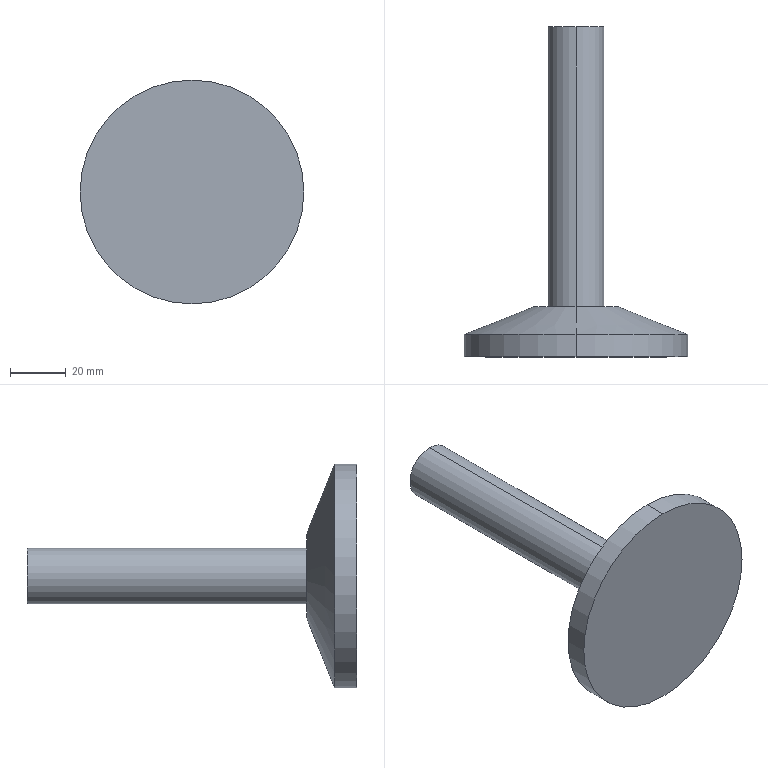Part | STEP file | 1 solid | 9 faces | box 80 x 118 x 80 mm | volume 97023 mm3 | cylinder 4 | plane 3 | cone 2 | commonest cylinder face diameters 20 x2 80 x2
STEP:
#1=CARTESIAN_POINT('',(0.,0.,0.));
#2=DIRECTION('',(0.,0.,1.));
#3=DIRECTION('',(1.,0.,0.));
#4=AXIS2_PLACEMENT_3D('',#1,#2,#3);
#5=CARTESIAN_POINT('',(0.,0.,40.));
#6=VERTEX_POINT('',#5);
#7=CARTESIAN_POINT('',(0.,0.,-40.));
#8=VERTEX_POINT('',#7);
#9=CARTESIAN_POINT('',(0.,0.,0.));
#10=DIRECTION('',(0.,1.,0.));
#11=DIRECTION('',(0.,0.,1.));
#12=AXIS2_PLACEMENT_3D('',#9,#10,#11);
#13=CIRCLE('',#12,40.);
#14=CARTESIAN_POINT('',(0.,0.,0.));
#15=DIRECTION('',(0.,1.,0.));
#16=DIRECTION('',(0.,0.,1.));
#17=AXIS2_PLACEMENT_3D('',#14,#15,#16);
#18=CYLINDRICAL_SURFACE('',#17,40.);
#19=CARTESIAN_POINT('',(0.,0.));
#20=DIRECTION('',(1.,0.));
#21=VECTOR('',#20,1.);
#22=LINE('',#19,#21);
#23=(GEOMETRIC_REPRESENTATION_CONTEXT(2)PARAMETRIC_REPRESENTATION_CONTEXT()REPRESENTATION_CONTEXT('',''));
#24=DEFINITIONAL_REPRESENTATION('',(#22),#23);
#25=PCURVE('',#18,#24);
#26=CARTESIAN_POINT('',(-40.,0.,0.));
#27=DIRECTION('',(0.,1.,0.));
#28=DIRECTION('',(0.,0.,1.));
#29=AXIS2_PLACEMENT_3D('',#26,#27,#28);
#30=PLANE('',#29);
#31=CARTESIAN_POINT('',(0.,40.));
#32=DIRECTION('',(1.,0.));
#33=AXIS2_PLACEMENT_2D('',#31,#32);
#34=CIRCLE('',#33,40.);
#35=(GEOMETRIC_REPRESENTATION_CONTEXT(2)PARAMETRIC_REPRESENTATION_CONTEXT()REPRESENTATION_CONTEXT('',''));
#36=DEFINITIONAL_REPRESENTATION('',(#34),#35);
#37=PCURVE('',#30,#36);
#38=SURFACE_CURVE('',#13,(#25,#37),.PCURVE_S1.);
#39=EDGE_CURVE('',#6,#8,#38,.T.);
#40=ORIENTED_EDGE('',*,*,#39,.T.);
#41=CARTESIAN_POINT('',(0.,8.,-40.));
#42=VERTEX_POINT('',#41);
#43=CARTESIAN_POINT('',(0.,0.,-40.));
#44=DIRECTION('',(0.,1.,0.));
#45=VECTOR('',#44,1.);
#46=LINE('',#43,#45);
#47=CARTESIAN_POINT('',(3.142,0.));
#48=DIRECTION('',(0.,1.));
#49=VECTOR('',#48,1.);
#50=LINE('',#47,#49);
#51=(GEOMETRIC_REPRESENTATION_CONTEXT(2)PARAMETRIC_REPRESENTATION_CONTEXT()REPRESENTATION_CONTEXT('',''));
#52=DEFINITIONAL_REPRESENTATION('',(#50),#51);
#53=PCURVE('',#18,#52);
#54=CARTESIAN_POINT('',(0.,0.,0.));
#55=DIRECTION('',(0.,1.,0.));
#56=DIRECTION('',(0.,0.,1.));
#57=AXIS2_PLACEMENT_3D('',#54,#55,#56);
#58=CYLINDRICAL_SURFACE('',#57,40.);
#59=CARTESIAN_POINT('',(3.142,0.));
#60=DIRECTION('',(0.,1.));
#61=VECTOR('',#60,1.);
#62=LINE('',#59,#61);
#63=(GEOMETRIC_REPRESENTATION_CONTEXT(2)PARAMETRIC_REPRESENTATION_CONTEXT()REPRESENTATION_CONTEXT('',''));
#64=DEFINITIONAL_REPRESENTATION('',(#62),#63);
#65=PCURVE('',#58,#64);
#66=SURFACE_CURVE('',#46,(#53,#65),.PCURVE_S1.);
#67=EDGE_CURVE('',#8,#42,#66,.T.);
#68=ORIENTED_EDGE('',*,*,#67,.T.);
#69=CARTESIAN_POINT('',(0.,8.,40.));
#70=VERTEX_POINT('',#69);
#71=CARTESIAN_POINT('',(0.,8.,0.));
#72=DIRECTION('',(0.,-1.,0.));
#73=DIRECTION('',(0.,0.,1.));
#74=AXIS2_PLACEMENT_3D('',#71,#72,#73);
#75=CIRCLE('',#74,40.);
#76=CARTESIAN_POINT('',(6.283,8.));
#77=DIRECTION('',(-1.,0.));
#78=VECTOR('',#77,1.);
#79=LINE('',#76,#78);
#80=(GEOMETRIC_REPRESENTATION_CONTEXT(2)PARAMETRIC_REPRESENTATION_CONTEXT()REPRESENTATION_CONTEXT('',''));
#81=DEFINITIONAL_REPRESENTATION('',(#79),#80);
#82=PCURVE('',#18,#81);
#83=CARTESIAN_POINT('',(0.,8.,0.));
#84=DIRECTION('',(0.,-1.,0.));
#85=DIRECTION('',(0.,0.,-1.));
#86=AXIS2_PLACEMENT_3D('',#83,#84,#85);
#87=CONICAL_SURFACE('',#86,40.,1.19);
#88=CARTESIAN_POINT('',(-3.142,0.));
#89=DIRECTION('',(1.,0.));
#90=VECTOR('',#89,1.);
#91=LINE('',#88,#90);
#92=(GEOMETRIC_REPRESENTATION_CONTEXT(2)PARAMETRIC_REPRESENTATION_CONTEXT()REPRESENTATION_CONTEXT('',''));
#93=DEFINITIONAL_REPRESENTATION('',(#91),#92);
#94=PCURVE('',#87,#93);
#95=SURFACE_CURVE('',#75,(#82,#94),.PCURVE_S1.);
#96=EDGE_CURVE('',#42,#70,#95,.T.);
#97=ORIENTED_EDGE('',*,*,#96,.T.);
#98=CARTESIAN_POINT('',(0.,0.,40.));
#99=DIRECTION('',(0.,1.,0.));
#100=VECTOR('',#99,1.);
#101=LINE('',#98,#100);
#102=CARTESIAN_POINT('',(0.,0.));
#103=DIRECTION('',(0.,1.));
#104=VECTOR('',#103,1.);
#105=LINE('',#102,#104);
#106=(GEOMETRIC_REPRESENTATION_CONTEXT(2)PARAMETRIC_REPRESENTATION_CONTEXT()REPRESENTATION_CONTEXT('',''));
#107=DEFINITIONAL_REPRESENTATION('',(#105),#106);
#108=PCURVE('',#18,#107);
#109=CARTESIAN_POINT('',(6.283,0.));
#110=DIRECTION('',(0.,1.));
#111=VECTOR('',#110,1.);
#112=LINE('',#109,#111);
#113=(GEOMETRIC_REPRESENTATION_CONTEXT(2)PARAMETRIC_REPRESENTATION_CONTEXT()REPRESENTATION_CONTEXT('',''));
#114=DEFINITIONAL_REPRESENTATION('',(#112),#113);
#115=PCURVE('',#58,#114);
#116=SURFACE_CURVE('',#101,(#108,#115),.PCURVE_S1.);
#117=EDGE_CURVE('',#6,#70,#116,.T.);
#118=ORIENTED_EDGE('',*,*,#117,.F.);
#119=EDGE_LOOP('',(#40,#68,#97,#118));
#120=FACE_BOUND('',#119,.T.);
#121=ADVANCED_FACE('',(#120),#18,.T.);
#122=CARTESIAN_POINT('',(0.,18.,-15.));
#123=VERTEX_POINT('',#122);
#124=CARTESIAN_POINT('',(0.,18.,15.));
#125=VERTEX_POINT('',#124);
#126=CARTESIAN_POINT('',(0.,18.,0.));
#127=DIRECTION('',(0.,-1.,0.));
#128=DIRECTION('',(0.,0.,-1.));
#129=AXIS2_PLACEMENT_3D('',#126,#127,#128);
#130=CIRCLE('',#129,15.);
#131=CARTESIAN_POINT('',(0.,-10.));
#132=DIRECTION('',(1.,0.));
#133=VECTOR('',#132,1.);
#134=LINE('',#131,#133);
#135=(GEOMETRIC_REPRESENTATION_CONTEXT(2)PARAMETRIC_REPRESENTATION_CONTEXT()REPRESENTATION_CONTEXT('',''));
#136=DEFINITIONAL_REPRESENTATION('',(#134),#135);
#137=PCURVE('',#87,#136);
#138=CARTESIAN_POINT('',(-10.,18.,0.));
#139=DIRECTION('',(0.,-1.,0.));
#140=DIRECTION('',(0.,0.,-1.));
#141=AXIS2_PLACEMENT_3D('',#138,#139,#140);
#142=PLANE('',#141);
#143=CARTESIAN_POINT('',(0.,10.));
#144=DIRECTION('',(1.,0.));
#145=AXIS2_PLACEMENT_2D('',#143,#144);
#146=CIRCLE('',#145,15.);
#147=(GEOMETRIC_REPRESENTATION_CONTEXT(2)PARAMETRIC_REPRESENTATION_CONTEXT()REPRESENTATION_CONTEXT('',''));
#148=DEFINITIONAL_REPRESENTATION('',(#146),#147);
#149=PCURVE('',#142,#148);
#150=SURFACE_CURVE('',#130,(#137,#149),.PCURVE_S1.);
#151=EDGE_CURVE('',#123,#125,#150,.T.);
#152=ORIENTED_EDGE('',*,*,#151,.T.);
#153=CARTESIAN_POINT('',(0.,8.,40.));
#154=DIRECTION('',(0.,-0.3714,0.9285));
#155=VECTOR('',#154,1.);
#156=LINE('',#153,#155);
#157=CARTESIAN_POINT('',(3.142,0.));
#158=DIRECTION('',(0.,1.));
#159=VECTOR('',#158,1.);
#160=LINE('',#157,#159);
#161=(GEOMETRIC_REPRESENTATION_CONTEXT(2)PARAMETRIC_REPRESENTATION_CONTEXT()REPRESENTATION_CONTEXT('',''));
#162=DEFINITIONAL_REPRESENTATION('',(#160),#161);
#163=PCURVE('',#87,#162);
#164=CARTESIAN_POINT('',(0.,8.,0.));
#165=DIRECTION('',(0.,-1.,0.));
#166=DIRECTION('',(0.,0.,-1.));
#167=AXIS2_PLACEMENT_3D('',#164,#165,#166);
#168=CONICAL_SURFACE('',#167,40.,1.19);
#169=CARTESIAN_POINT('',(3.142,0.));
#170=DIRECTION('',(0.,1.));
#171=VECTOR('',#170,1.);
#172=LINE('',#169,#171);
#173=(GEOMETRIC_REPRESENTATION_CONTEXT(2)PARAMETRIC_REPRESENTATION_CONTEXT()REPRESENTATION_CONTEXT('',''));
#174=DEFINITIONAL_REPRESENTATION('',(#172),#173);
#175=PCURVE('',#168,#174);
#176=SURFACE_CURVE('',#156,(#163,#175),.PCURVE_S1.);
#177=EDGE_CURVE('',#125,#70,#176,.T.);
#178=ORIENTED_EDGE('',*,*,#177,.T.);
#179=ORIENTED_EDGE('',*,*,#96,.F.);
#180=CARTESIAN_POINT('',(0.,8.,-40.));
#181=DIRECTION('',(0.,-0.3714,-0.9285));
#182=VECTOR('',#181,1.);
#183=LINE('',#180,#182);
#184=CARTESIAN_POINT('',(0.,0.));
#185=DIRECTION('',(0.,1.));
#186=VECTOR('',#185,1.);
#187=LINE('',#184,#186);
#188=(GEOMETRIC_REPRESENTATION_CONTEXT(2)PARAMETRIC_REPRESENTATION_CONTEXT()REPRESENTATION_CONTEXT('',''));
#189=DEFINITIONAL_REPRESENTATION('',(#187),#188);
#190=PCURVE('',#87,#189);
#191=CARTESIAN_POINT('',(6.283,0.));
#192=DIRECTION('',(0.,1.));
#193=VECTOR('',#192,1.);
#194=LINE('',#191,#193);
#195=(GEOMETRIC_REPRESENTATION_CONTEXT(2)PARAMETRIC_REPRESENTATION_CONTEXT()REPRESENTATION_CONTEXT('',''));
#196=DEFINITIONAL_REPRESENTATION('',(#194),#195);
#197=PCURVE('',#168,#196);
#198=SURFACE_CURVE('',#183,(#190,#197),.PCURVE_S1.);
#199=EDGE_CURVE('',#123,#42,#198,.T.);
#200=ORIENTED_EDGE('',*,*,#199,.F.);
#201=EDGE_LOOP('',(#152,#178,#179,#200));
#202=FACE_BOUND('',#201,.T.);
#203=ADVANCED_FACE('',(#202),#87,.T.);
#204=CARTESIAN_POINT('',(0.,18.,10.));
#205=VERTEX_POINT('',#204);
#206=CARTESIAN_POINT('',(0.,18.,-10.));
#207=VERTEX_POINT('',#206);
#208=CARTESIAN_POINT('',(0.,18.,0.));
#209=DIRECTION('',(0.,1.,0.));
#210=DIRECTION('',(0.,0.,1.));
#211=AXIS2_PLACEMENT_3D('',#208,#209,#210);
#212=CIRCLE('',#211,10.);
#213=CARTESIAN_POINT('',(0.,0.,0.));
#214=DIRECTION('',(0.,1.,0.));
#215=DIRECTION('',(0.,0.,1.));
#216=AXIS2_PLACEMENT_3D('',#213,#214,#215);
#217=CYLINDRICAL_SURFACE('',#216,10.);
#218=CARTESIAN_POINT('',(0.,18.));
#219=DIRECTION('',(1.,0.));
#220=VECTOR('',#219,1.);
#221=LINE('',#218,#220);
#222=(GEOMETRIC_REPRESENTATION_CONTEXT(2)PARAMETRIC_REPRESENTATION_CONTEXT()REPRESENTATION_CONTEXT('',''));
#223=DEFINITIONAL_REPRESENTATION('',(#221),#222);
#224=PCURVE('',#217,#223);
#225=CARTESIAN_POINT('',(-10.,10.));
#226=CARTESIAN_POINT('',(-10.,27.321));
#227=CARTESIAN_POINT('',(5.,18.66));
#228=CARTESIAN_POINT('',(20.,10.));
#229=CARTESIAN_POINT('',(5.,1.34));
#230=CARTESIAN_POINT('',(-10.,-7.321));
#231=CARTESIAN_POINT('',(-10.,10.));
#232=(BOUNDED_CURVE()B_SPLINE_CURVE(2,(#225,#226,#227,#228,#229,#230,#231),.UNSPECIFIED.,.T.,.F.)B_SPLINE_CURVE_WITH_KNOTS((1,2,2,2,2,1),(-2.094,0.,2.094,4.189,6.283,8.378),.UNSPECIFIED.)CURVE()GEOMETRIC_REPRESENTATION_ITEM()RATIONAL_B_SPLINE_CURVE((1.,0.5,1.,0.5,1.,0.5,1.))REPRESENTATION_ITEM(''));
#233=(GEOMETRIC_REPRESENTATION_CONTEXT(2)PARAMETRIC_REPRESENTATION_CONTEXT()REPRESENTATION_CONTEXT('',''));
#234=DEFINITIONAL_REPRESENTATION('',(#232),#233);
#235=PCURVE('',#142,#234);
#236=SURFACE_CURVE('',#212,(#224,#235),.PCURVE_S1.);
#237=EDGE_CURVE('',#205,#207,#236,.T.);
#238=ORIENTED_EDGE('',*,*,#237,.T.);
#239=CARTESIAN_POINT('',(0.,118.,-10.));
#240=VERTEX_POINT('',#239);
#241=CARTESIAN_POINT('',(0.,0.,-10.));
#242=DIRECTION('',(0.,1.,0.));
#243=VECTOR('',#242,1.);
#244=LINE('',#241,#243);
#245=CARTESIAN_POINT('',(3.142,0.));
#246=DIRECTION('',(0.,1.));
#247=VECTOR('',#246,1.);
#248=LINE('',#245,#247);
#249=(GEOMETRIC_REPRESENTATION_CONTEXT(2)PARAMETRIC_REPRESENTATION_CONTEXT()REPRESENTATION_CONTEXT('',''));
#250=DEFINITIONAL_REPRESENTATION('',(#248),#249);
#251=PCURVE('',#217,#250);
#252=CARTESIAN_POINT('',(0.,0.,0.));
#253=DIRECTION('',(0.,1.,0.));
#254=DIRECTION('',(0.,0.,1.));
#255=AXIS2_PLACEMENT_3D('',#252,#253,#254);
#256=CYLINDRICAL_SURFACE('',#255,10.);
#257=CARTESIAN_POINT('',(3.142,0.));
#258=DIRECTION('',(0.,1.));
#259=VECTOR('',#258,1.);
#260=LINE('',#257,#259);
#261=(GEOMETRIC_REPRESENTATION_CONTEXT(2)PARAMETRIC_REPRESENTATION_CONTEXT()REPRESENTATION_CONTEXT('',''));
#262=DEFINITIONAL_REPRESENTATION('',(#260),#261);
#263=PCURVE('',#256,#262);
#264=SURFACE_CURVE('',#244,(#251,#263),.PCURVE_S1.);
#265=EDGE_CURVE('',#207,#240,#264,.T.);
#266=ORIENTED_EDGE('',*,*,#265,.T.);
#267=CARTESIAN_POINT('',(0.,118.,10.));
#268=VERTEX_POINT('',#267);
#269=CARTESIAN_POINT('',(0.,118.,0.));
#270=DIRECTION('',(0.,-1.,0.));
#271=DIRECTION('',(0.,0.,1.));
#272=AXIS2_PLACEMENT_3D('',#269,#270,#271);
#273=CIRCLE('',#272,10.);
#274=CARTESIAN_POINT('',(6.283,118.));
#275=DIRECTION('',(-1.,0.));
#276=VECTOR('',#275,1.);
#277=LINE('',#274,#276);
#278=(GEOMETRIC_REPRESENTATION_CONTEXT(2)PARAMETRIC_REPRESENTATION_CONTEXT()REPRESENTATION_CONTEXT('',''));
#279=DEFINITIONAL_REPRESENTATION('',(#277),#278);
#280=PCURVE('',#217,#279);
#281=CARTESIAN_POINT('',(0.,118.,0.));
#282=DIRECTION('',(0.,-1.,0.));
#283=DIRECTION('',(0.,0.,-1.));
#284=AXIS2_PLACEMENT_3D('',#281,#282,#283);
#285=PLANE('',#284);
#286=CARTESIAN_POINT('',(0.,0.));
#287=DIRECTION('',(-1.,0.));
#288=AXIS2_PLACEMENT_2D('',#286,#287);
#289=CIRCLE('',#288,10.);
#290=(GEOMETRIC_REPRESENTATION_CONTEXT(2)PARAMETRIC_REPRESENTATION_CONTEXT()REPRESENTATION_CONTEXT('',''));
#291=DEFINITIONAL_REPRESENTATION('',(#289),#290);
#292=PCURVE('',#285,#291);
#293=SURFACE_CURVE('',#273,(#280,#292),.PCURVE_S1.);
#294=EDGE_CURVE('',#240,#268,#293,.T.);
#295=ORIENTED_EDGE('',*,*,#294,.T.);
#296=CARTESIAN_POINT('',(0.,0.,10.));
#297=DIRECTION('',(0.,1.,0.));
#298=VECTOR('',#297,1.);
#299=LINE('',#296,#298);
#300=CARTESIAN_POINT('',(0.,0.));
#301=DIRECTION('',(0.,1.));
#302=VECTOR('',#301,1.);
#303=LINE('',#300,#302);
#304=(GEOMETRIC_REPRESENTATION_CONTEXT(2)PARAMETRIC_REPRESENTATION_CONTEXT()REPRESENTATION_CONTEXT('',''));
#305=DEFINITIONAL_REPRESENTATION('',(#303),#304);
#306=PCURVE('',#217,#305);
#307=CARTESIAN_POINT('',(6.283,0.));
#308=DIRECTION('',(0.,1.));
#309=VECTOR('',#308,1.);
#310=LINE('',#307,#309);
#311=(GEOMETRIC_REPRESENTATION_CONTEXT(2)PARAMETRIC_REPRESENTATION_CONTEXT()REPRESENTATION_CONTEXT('',''));
#312=DEFINITIONAL_REPRESENTATION('',(#310),#311);
#313=PCURVE('',#256,#312);
#314=SURFACE_CURVE('',#299,(#306,#313),.PCURVE_S1.);
#315=EDGE_CURVE('',#205,#268,#314,.T.);
#316=ORIENTED_EDGE('',*,*,#315,.F.);
#317=EDGE_LOOP('',(#238,#266,#295,#316));
#318=FACE_BOUND('',#317,.T.);
#319=ADVANCED_FACE('',(#318),#217,.T.);
#320=ORIENTED_EDGE('',*,*,#39,.F.);
#321=CARTESIAN_POINT('',(0.,0.,0.));
#322=DIRECTION('',(0.,1.,0.));
#323=DIRECTION('',(0.,0.,1.));
#324=AXIS2_PLACEMENT_3D('',#321,#322,#323);
#325=CIRCLE('',#324,40.);
#326=CARTESIAN_POINT('',(0.,40.));
#327=DIRECTION('',(1.,0.));
#328=AXIS2_PLACEMENT_2D('',#326,#327);
#329=CIRCLE('',#328,40.);
#330=(GEOMETRIC_REPRESENTATION_CONTEXT(2)PARAMETRIC_REPRESENTATION_CONTEXT()REPRESENTATION_CONTEXT('',''));
#331=DEFINITIONAL_REPRESENTATION('',(#329),#330);
#332=PCURVE('',#30,#331);
#333=CARTESIAN_POINT('',(0.,0.));
#334=DIRECTION('',(1.,0.));
#335=VECTOR('',#334,1.);
#336=LINE('',#333,#335);
#337=(GEOMETRIC_REPRESENTATION_CONTEXT(2)PARAMETRIC_REPRESENTATION_CONTEXT()REPRESENTATION_CONTEXT('',''));
#338=DEFINITIONAL_REPRESENTATION('',(#336),#337);
#339=PCURVE('',#58,#338);
#340=SURFACE_CURVE('',#325,(#332,#339),.PCURVE_S1.);
#341=EDGE_CURVE('',#8,#6,#340,.T.);
#342=ORIENTED_EDGE('',*,*,#341,.F.);
#343=EDGE_LOOP('',(#320,#342));
#344=FACE_BOUND('',#343,.T.);
#345=ADVANCED_FACE('',(#344),#30,.F.);
#346=ORIENTED_EDGE('',*,*,#67,.F.);
#347=ORIENTED_EDGE('',*,*,#341,.T.);
#348=ORIENTED_EDGE('',*,*,#117,.T.);
#349=CARTESIAN_POINT('',(0.,8.,0.));
#350=DIRECTION('',(0.,-1.,0.));
#351=DIRECTION('',(0.,0.,1.));
#352=AXIS2_PLACEMENT_3D('',#349,#350,#351);
#353=CIRCLE('',#352,40.);
#354=CARTESIAN_POINT('',(6.283,8.));
#355=DIRECTION('',(-1.,0.));
#356=VECTOR('',#355,1.);
#357=LINE('',#354,#356);
#358=(GEOMETRIC_REPRESENTATION_CONTEXT(2)PARAMETRIC_REPRESENTATION_CONTEXT()REPRESENTATION_CONTEXT('',''));
#359=DEFINITIONAL_REPRESENTATION('',(#357),#358);
#360=PCURVE('',#58,#359);
#361=CARTESIAN_POINT('',(3.142,0.));
#362=DIRECTION('',(1.,0.));
#363=VECTOR('',#362,1.);
#364=LINE('',#361,#363);
#365=(GEOMETRIC_REPRESENTATION_CONTEXT(2)PARAMETRIC_REPRESENTATION_CONTEXT()REPRESENTATION_CONTEXT('',''));
#366=DEFINITIONAL_REPRESENTATION('',(#364),#365);
#367=PCURVE('',#168,#366);
#368=SURFACE_CURVE('',#353,(#360,#367),.PCURVE_S1.);
#369=EDGE_CURVE('',#70,#42,#368,.T.);
#370=ORIENTED_EDGE('',*,*,#369,.T.);
#371=EDGE_LOOP('',(#346,#347,#348,#370));
#372=FACE_BOUND('',#371,.T.);
#373=ADVANCED_FACE('',(#372),#58,.T.);
#374=ORIENTED_EDGE('',*,*,#177,.F.);
#375=CARTESIAN_POINT('',(0.,18.,0.));
#376=DIRECTION('',(0.,-1.,0.));
#377=DIRECTION('',(0.,0.,-1.));
#378=AXIS2_PLACEMENT_3D('',#375,#376,#377);
#379=CIRCLE('',#378,15.);
#380=CARTESIAN_POINT('',(0.,-10.));
#381=DIRECTION('',(1.,0.));
#382=VECTOR('',#381,1.);
#383=LINE('',#380,#382);
#384=(GEOMETRIC_REPRESENTATION_CONTEXT(2)PARAMETRIC_REPRESENTATION_CONTEXT()REPRESENTATION_CONTEXT('',''));
#385=DEFINITIONAL_REPRESENTATION('',(#383),#384);
#386=PCURVE('',#168,#385);
#387=CARTESIAN_POINT('',(0.,10.));
#388=DIRECTION('',(1.,0.));
#389=AXIS2_PLACEMENT_2D('',#387,#388);
#390=CIRCLE('',#389,15.);
#391=(GEOMETRIC_REPRESENTATION_CONTEXT(2)PARAMETRIC_REPRESENTATION_CONTEXT()REPRESENTATION_CONTEXT('',''));
#392=DEFINITIONAL_REPRESENTATION('',(#390),#391);
#393=PCURVE('',#142,#392);
#394=SURFACE_CURVE('',#379,(#386,#393),.PCURVE_S1.);
#395=EDGE_CURVE('',#125,#123,#394,.T.);
#396=ORIENTED_EDGE('',*,*,#395,.T.);
#397=ORIENTED_EDGE('',*,*,#199,.T.);
#398=ORIENTED_EDGE('',*,*,#369,.F.);
#399=EDGE_LOOP('',(#374,#396,#397,#398));
#400=FACE_BOUND('',#399,.T.);
#401=ADVANCED_FACE('',(#400),#168,.T.);
#402=ORIENTED_EDGE('',*,*,#237,.F.);
#403=CARTESIAN_POINT('',(0.,18.,0.));
#404=DIRECTION('',(0.,1.,0.));
#405=DIRECTION('',(0.,0.,1.));
#406=AXIS2_PLACEMENT_3D('',#403,#404,#405);
#407=CIRCLE('',#406,10.);
#408=CARTESIAN_POINT('',(-10.,10.));
#409=CARTESIAN_POINT('',(-10.,27.321));
#410=CARTESIAN_POINT('',(5.,18.66));
#411=CARTESIAN_POINT('',(20.,10.));
#412=CARTESIAN_POINT('',(5.,1.34));
#413=CARTESIAN_POINT('',(-10.,-7.321));
#414=CARTESIAN_POINT('',(-10.,10.));
#415=(BOUNDED_CURVE()B_SPLINE_CURVE(2,(#408,#409,#410,#411,#412,#413,#414),.UNSPECIFIED.,.T.,.F.)B_SPLINE_CURVE_WITH_KNOTS((1,2,2,2,2,1),(-2.094,0.,2.094,4.189,6.283,8.378),.UNSPECIFIED.)CURVE()GEOMETRIC_REPRESENTATION_ITEM()RATIONAL_B_SPLINE_CURVE((1.,0.5,1.,0.5,1.,0.5,1.))REPRESENTATION_ITEM(''));
#416=(GEOMETRIC_REPRESENTATION_CONTEXT(2)PARAMETRIC_REPRESENTATION_CONTEXT()REPRESENTATION_CONTEXT('',''));
#417=DEFINITIONAL_REPRESENTATION('',(#415),#416);
#418=PCURVE('',#142,#417);
#419=CARTESIAN_POINT('',(0.,18.));
#420=DIRECTION('',(1.,0.));
#421=VECTOR('',#420,1.);
#422=LINE('',#419,#421);
#423=(GEOMETRIC_REPRESENTATION_CONTEXT(2)PARAMETRIC_REPRESENTATION_CONTEXT()REPRESENTATION_CONTEXT('',''));
#424=DEFINITIONAL_REPRESENTATION('',(#422),#423);
#425=PCURVE('',#256,#424);
#426=SURFACE_CURVE('',#407,(#418,#425),.PCURVE_S1.);
#427=EDGE_CURVE('',#207,#205,#426,.T.);
#428=ORIENTED_EDGE('',*,*,#427,.F.);
#429=EDGE_LOOP('',(#402,#428));
#430=FACE_BOUND('',#429,.T.);
#431=ORIENTED_EDGE('',*,*,#151,.F.);
#432=ORIENTED_EDGE('',*,*,#395,.F.);
#433=EDGE_LOOP('',(#431,#432));
#434=FACE_BOUND('',#433,.T.);
#435=ADVANCED_FACE('',(#430,#434),#142,.F.);
#436=ORIENTED_EDGE('',*,*,#265,.F.);
#437=ORIENTED_EDGE('',*,*,#427,.T.);
#438=ORIENTED_EDGE('',*,*,#315,.T.);
#439=CARTESIAN_POINT('',(0.,118.,0.));
#440=DIRECTION('',(0.,-1.,0.));
#441=DIRECTION('',(0.,0.,1.));
#442=AXIS2_PLACEMENT_3D('',#439,#440,#441);
#443=CIRCLE('',#442,10.);
#444=CARTESIAN_POINT('',(6.283,118.));
#445=DIRECTION('',(-1.,0.));
#446=VECTOR('',#445,1.);
#447=LINE('',#444,#446);
#448=(GEOMETRIC_REPRESENTATION_CONTEXT(2)PARAMETRIC_REPRESENTATION_CONTEXT()REPRESENTATION_CONTEXT('',''));
#449=DEFINITIONAL_REPRESENTATION('',(#447),#448);
#450=PCURVE('',#256,#449);
#451=CARTESIAN_POINT('',(0.,0.));
#452=DIRECTION('',(-1.,0.));
#453=AXIS2_PLACEMENT_2D('',#451,#452);
#454=CIRCLE('',#453,10.);
#455=(GEOMETRIC_REPRESENTATION_CONTEXT(2)PARAMETRIC_REPRESENTATION_CONTEXT()REPRESENTATION_CONTEXT('',''));
#456=DEFINITIONAL_REPRESENTATION('',(#454),#455);
#457=PCURVE('',#285,#456);
#458=SURFACE_CURVE('',#443,(#450,#457),.PCURVE_S1.);
#459=EDGE_CURVE('',#268,#240,#458,.T.);
#460=ORIENTED_EDGE('',*,*,#459,.T.);
#461=EDGE_LOOP('',(#436,#437,#438,#460));
#462=FACE_BOUND('',#461,.T.);
#463=ADVANCED_FACE('',(#462),#256,.T.);
#464=ORIENTED_EDGE('',*,*,#459,.F.);
#465=ORIENTED_EDGE('',*,*,#294,.F.);
#466=EDGE_LOOP('',(#464,#465));
#467=FACE_BOUND('',#466,.T.);
#468=ADVANCED_FACE('',(#467),#285,.F.);
#469=CLOSED_SHELL('',(#121,#203,#319,#345,#373,#401,#435,#463,#468));
#470=MANIFOLD_SOLID_BREP('',#469);
#471=(LENGTH_UNIT()NAMED_UNIT(*)SI_UNIT(.MILLI.,.METRE.));
#472=UNCERTAINTY_MEASURE_WITH_UNIT(LENGTH_MEASURE(0.0000001),#471,'','');
#473=(NAMED_UNIT(*)PLANE_ANGLE_UNIT()SI_UNIT($,.RADIAN.));
#474=(NAMED_UNIT(*)SI_UNIT($,.STERADIAN.)SOLID_ANGLE_UNIT());
#475=(GEOMETRIC_REPRESENTATION_CONTEXT(3)GLOBAL_UNCERTAINTY_ASSIGNED_CONTEXT((#472))GLOBAL_UNIT_ASSIGNED_CONTEXT((#471,#473,#474))REPRESENTATION_CONTEXT('',''));
#476=ADVANCED_BREP_SHAPE_REPRESENTATION('',(#4,#470),#475);